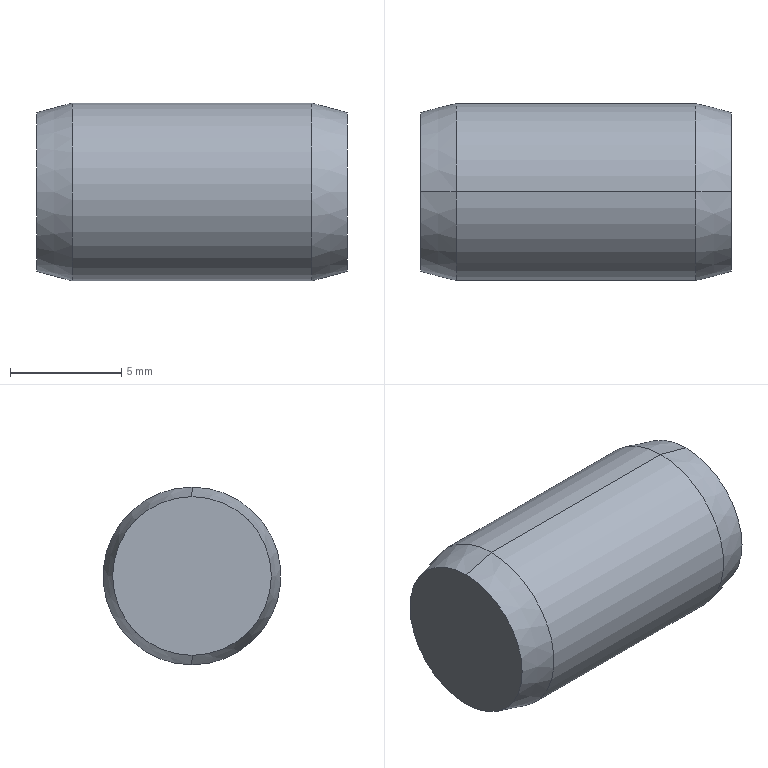Part | SolidWorks | features Revolution 1 | 1 solid | 8 faces | box 14 x 8 x 8 mm | volume 687.093 mm3 | cone 4 | cylinder 2 | plane 2 | commonest cylinder face diameters 8 x2
STEP:
#1=CARTESIAN_POINT('',(0.,0.,3.571));
#2=VERTEX_POINT('',#1);
#3=CARTESIAN_POINT('',(0.,0.,-3.571));
#4=VERTEX_POINT('',#3);
#5=CARTESIAN_POINT('',(0.,0.,0.));
#6=DIRECTION('',(-1.,0.,0.));
#7=DIRECTION('',(0.,0.,1.));
#8=AXIS2_PLACEMENT_3D('',#5,#6,#7);
#9=CIRCLE('',#8,3.571);
#10=EDGE_CURVE('',#2,#4,#9,.T.);
#11=ORIENTED_EDGE('',*,*,#10,.F.);
#12=CARTESIAN_POINT('',(1.6,0.,4.));
#13=VERTEX_POINT('',#12);
#14=CARTESIAN_POINT('',(1.6,0.,4.));
#15=DIRECTION('',(0.9659,0.,0.2588));
#16=VECTOR('',#15,1000.);
#17=LINE('',#14,#16);
#18=EDGE_CURVE('',#2,#13,#17,.T.);
#19=ORIENTED_EDGE('',*,*,#18,.T.);
#20=CARTESIAN_POINT('',(1.6,0.,-4.));
#21=VERTEX_POINT('',#20);
#22=CARTESIAN_POINT('',(1.6,0.,0.));
#23=DIRECTION('',(-1.,0.,0.));
#24=DIRECTION('',(0.,0.,1.));
#25=AXIS2_PLACEMENT_3D('',#22,#23,#24);
#26=CIRCLE('',#25,4.);
#27=EDGE_CURVE('',#13,#21,#26,.T.);
#28=ORIENTED_EDGE('',*,*,#27,.T.);
#29=CARTESIAN_POINT('',(1.6,0.,-4.));
#30=DIRECTION('',(0.9659,0.,-0.2588));
#31=VECTOR('',#30,1000.);
#32=LINE('',#29,#31);
#33=EDGE_CURVE('',#4,#21,#32,.T.);
#34=ORIENTED_EDGE('',*,*,#33,.F.);
#35=EDGE_LOOP('',(#11,#19,#28,#34));
#36=FACE_OUTER_BOUND('',#35,.T.);
#37=CARTESIAN_POINT('',(1.6,0.,0.));
#38=DIRECTION('',(1.,0.,0.));
#39=DIRECTION('',(0.,0.,-1.));
#40=AXIS2_PLACEMENT_3D('',#37,#38,#39);
#41=CONICAL_SURFACE('',#40,4.,0.2618);
#42=ADVANCED_FACE('',(#36),#41,.T.);
#43=CARTESIAN_POINT('',(12.4,0.,4.));
#44=VERTEX_POINT('',#43);
#45=CARTESIAN_POINT('',(12.4,0.,-4.));
#46=VERTEX_POINT('',#45);
#47=CARTESIAN_POINT('',(12.4,0.,0.));
#48=DIRECTION('',(-1.,0.,0.));
#49=DIRECTION('',(0.,0.,1.));
#50=AXIS2_PLACEMENT_3D('',#47,#48,#49);
#51=CIRCLE('',#50,4.);
#52=EDGE_CURVE('',#44,#46,#51,.T.);
#53=ORIENTED_EDGE('',*,*,#52,.T.);
#54=CARTESIAN_POINT('',(-1.656,0.,-4.));
#55=DIRECTION('',(-1.,0.,0.));
#56=VECTOR('',#55,1000.);
#57=LINE('',#54,#56);
#58=EDGE_CURVE('',#46,#21,#57,.T.);
#59=ORIENTED_EDGE('',*,*,#58,.T.);
#60=ORIENTED_EDGE('',*,*,#27,.F.);
#61=CARTESIAN_POINT('',(-1.656,0.,4.));
#62=DIRECTION('',(-1.,0.,0.));
#63=VECTOR('',#62,1000.);
#64=LINE('',#61,#63);
#65=EDGE_CURVE('',#44,#13,#64,.T.);
#66=ORIENTED_EDGE('',*,*,#65,.F.);
#67=EDGE_LOOP('',(#53,#59,#60,#66));
#68=FACE_OUTER_BOUND('',#67,.T.);
#69=CARTESIAN_POINT('',(-1.656,0.,0.));
#70=DIRECTION('',(-1.,0.,0.));
#71=DIRECTION('',(0.,0.,1.));
#72=AXIS2_PLACEMENT_3D('',#69,#70,#71);
#73=CYLINDRICAL_SURFACE('',#72,4.);
#74=ADVANCED_FACE('',(#68),#73,.T.);
#75=CARTESIAN_POINT('',(14.,0.,3.571));
#76=VERTEX_POINT('',#75);
#77=CARTESIAN_POINT('',(14.,0.,-3.571));
#78=VERTEX_POINT('',#77);
#79=CARTESIAN_POINT('',(14.,0.,0.));
#80=DIRECTION('',(-1.,0.,0.));
#81=DIRECTION('',(0.,0.,1.));
#82=AXIS2_PLACEMENT_3D('',#79,#80,#81);
#83=CIRCLE('',#82,3.571);
#84=EDGE_CURVE('',#76,#78,#83,.T.);
#85=ORIENTED_EDGE('',*,*,#84,.T.);
#86=CARTESIAN_POINT('',(14.,0.,-3.571));
#87=DIRECTION('',(-0.9659,0.,-0.2588));
#88=VECTOR('',#87,1000.);
#89=LINE('',#86,#88);
#90=EDGE_CURVE('',#78,#46,#89,.T.);
#91=ORIENTED_EDGE('',*,*,#90,.T.);
#92=ORIENTED_EDGE('',*,*,#52,.F.);
#93=CARTESIAN_POINT('',(14.,0.,3.571));
#94=DIRECTION('',(-0.9659,0.,0.2588));
#95=VECTOR('',#94,1000.);
#96=LINE('',#93,#95);
#97=EDGE_CURVE('',#76,#44,#96,.T.);
#98=ORIENTED_EDGE('',*,*,#97,.F.);
#99=EDGE_LOOP('',(#85,#91,#92,#98));
#100=FACE_OUTER_BOUND('',#99,.T.);
#101=CARTESIAN_POINT('',(14.,0.,0.));
#102=DIRECTION('',(-1.,0.,0.));
#103=DIRECTION('',(0.,0.,1.));
#104=AXIS2_PLACEMENT_3D('',#101,#102,#103);
#105=CONICAL_SURFACE('',#104,3.571,0.2618);
#106=ADVANCED_FACE('',(#100),#105,.T.);
#107=CARTESIAN_POINT('',(0.,0.,0.));
#108=DIRECTION('',(-1.,0.,0.));
#109=DIRECTION('',(0.,0.,1.));
#110=AXIS2_PLACEMENT_3D('',#107,#108,#109);
#111=CIRCLE('',#110,3.571);
#112=EDGE_CURVE('',#4,#2,#111,.T.);
#113=ORIENTED_EDGE('',*,*,#112,.T.);
#114=ORIENTED_EDGE('',*,*,#10,.T.);
#115=EDGE_LOOP('',(#113,#114));
#116=FACE_OUTER_BOUND('',#115,.T.);
#117=CARTESIAN_POINT('',(0.,3.571,0.));
#118=DIRECTION('',(1.,0.,0.));
#119=DIRECTION('',(0.,0.,-1.));
#120=AXIS2_PLACEMENT_3D('',#117,#118,#119);
#121=PLANE('',#120);
#122=ADVANCED_FACE('',(#116),#121,.F.);
#123=ORIENTED_EDGE('',*,*,#84,.F.);
#124=CARTESIAN_POINT('',(14.,0.,0.));
#125=DIRECTION('',(-1.,0.,0.));
#126=DIRECTION('',(0.,0.,1.));
#127=AXIS2_PLACEMENT_3D('',#124,#125,#126);
#128=CIRCLE('',#127,3.571);
#129=EDGE_CURVE('',#78,#76,#128,.T.);
#130=ORIENTED_EDGE('',*,*,#129,.F.);
#131=EDGE_LOOP('',(#123,#130));
#132=FACE_OUTER_BOUND('',#131,.T.);
#133=CARTESIAN_POINT('',(14.,0.,0.));
#134=DIRECTION('',(-1.,0.,0.));
#135=DIRECTION('',(0.,0.,1.));
#136=AXIS2_PLACEMENT_3D('',#133,#134,#135);
#137=PLANE('',#136);
#138=ADVANCED_FACE('',(#132),#137,.F.);
#139=ORIENTED_EDGE('',*,*,#90,.F.);
#140=ORIENTED_EDGE('',*,*,#129,.T.);
#141=ORIENTED_EDGE('',*,*,#97,.T.);
#142=CARTESIAN_POINT('',(12.4,0.,0.));
#143=DIRECTION('',(-1.,0.,0.));
#144=DIRECTION('',(0.,0.,1.));
#145=AXIS2_PLACEMENT_3D('',#142,#143,#144);
#146=CIRCLE('',#145,4.);
#147=EDGE_CURVE('',#46,#44,#146,.T.);
#148=ORIENTED_EDGE('',*,*,#147,.F.);
#149=EDGE_LOOP('',(#139,#140,#141,#148));
#150=FACE_OUTER_BOUND('',#149,.T.);
#151=CARTESIAN_POINT('',(14.,0.,0.));
#152=DIRECTION('',(-1.,0.,0.));
#153=DIRECTION('',(0.,0.,1.));
#154=AXIS2_PLACEMENT_3D('',#151,#152,#153);
#155=CONICAL_SURFACE('',#154,3.571,0.2618);
#156=ADVANCED_FACE('',(#150),#155,.T.);
#157=ORIENTED_EDGE('',*,*,#58,.F.);
#158=ORIENTED_EDGE('',*,*,#147,.T.);
#159=ORIENTED_EDGE('',*,*,#65,.T.);
#160=CARTESIAN_POINT('',(1.6,0.,0.));
#161=DIRECTION('',(-1.,0.,0.));
#162=DIRECTION('',(0.,0.,1.));
#163=AXIS2_PLACEMENT_3D('',#160,#161,#162);
#164=CIRCLE('',#163,4.);
#165=EDGE_CURVE('',#21,#13,#164,.T.);
#166=ORIENTED_EDGE('',*,*,#165,.F.);
#167=EDGE_LOOP('',(#157,#158,#159,#166));
#168=FACE_OUTER_BOUND('',#167,.T.);
#169=CARTESIAN_POINT('',(-1.656,0.,0.));
#170=DIRECTION('',(-1.,0.,0.));
#171=DIRECTION('',(0.,0.,1.));
#172=AXIS2_PLACEMENT_3D('',#169,#170,#171);
#173=CYLINDRICAL_SURFACE('',#172,4.);
#174=ADVANCED_FACE('',(#168),#173,.T.);
#175=ORIENTED_EDGE('',*,*,#18,.F.);
#176=ORIENTED_EDGE('',*,*,#112,.F.);
#177=ORIENTED_EDGE('',*,*,#33,.T.);
#178=ORIENTED_EDGE('',*,*,#165,.T.);
#179=EDGE_LOOP('',(#175,#176,#177,#178));
#180=FACE_OUTER_BOUND('',#179,.T.);
#181=CARTESIAN_POINT('',(1.6,0.,0.));
#182=DIRECTION('',(1.,0.,0.));
#183=DIRECTION('',(0.,0.,-1.));
#184=AXIS2_PLACEMENT_3D('',#181,#182,#183);
#185=CONICAL_SURFACE('',#184,4.,0.2618);
#186=ADVANCED_FACE('',(#180),#185,.T.);
#187=CLOSED_SHELL('',(#42,#74,#106,#122,#138,#156,#174,#186));
#188=MANIFOLD_SOLID_BREP('',#187);
#189=CARTESIAN_POINT('',(0.,0.,0.));
#190=DIRECTION('',(0.,0.,1.));
#191=DIRECTION('',(1.,0.,0.));
#192=AXIS2_PLACEMENT_3D('',#189,#190,#191);
#193=(LENGTH_UNIT()NAMED_UNIT(*)SI_UNIT(.MILLI.,.METRE.));
#194=UNCERTAINTY_MEASURE_WITH_UNIT(LENGTH_MEASURE(0.00001),#193,'','');
#195=(NAMED_UNIT(*)PLANE_ANGLE_UNIT()SI_UNIT($,.RADIAN.));
#196=(NAMED_UNIT(*)SI_UNIT($,.STERADIAN.)SOLID_ANGLE_UNIT());
#197=(GEOMETRIC_REPRESENTATION_CONTEXT(3)GLOBAL_UNCERTAINTY_ASSIGNED_CONTEXT((#194))GLOBAL_UNIT_ASSIGNED_CONTEXT((#193,#195,#196))REPRESENTATION_CONTEXT('',''));
#198=ADVANCED_BREP_SHAPE_REPRESENTATION('',(#188,#192),#197);